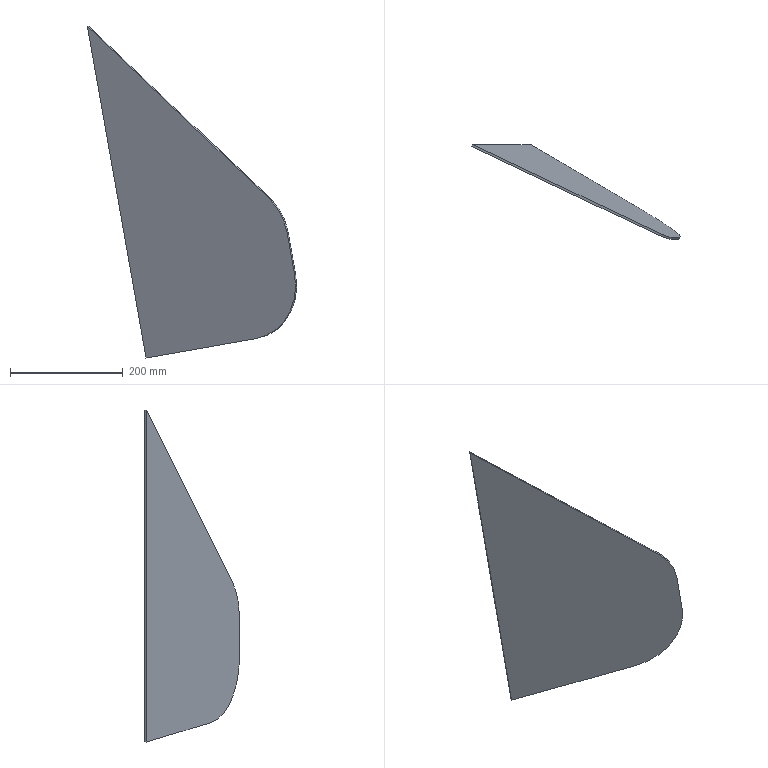Part | STEP file | floating channel left front section | 1 solid | 8 faces | box 372.026 x 168.494 x 590.246 mm | volume 526748 mm3 | plane 6 | cylinder 2 | commonest cylinder face diameters 200 x2
STEP:
#1=CARTESIAN_POINT('',(0.,0.,0.));
#2=DIRECTION('',(0.,0.,1.));
#3=DIRECTION('',(1.,0.,0.));
#4=AXIS2_PLACEMENT_3D('',#1,#2,#3);
#5=CARTESIAN_POINT('',(2326.268,155.426,-236.438));
#6=VERTEX_POINT('',#5);
#7=CARTESIAN_POINT('',(2358.025,143.435,-296.806));
#8=VERTEX_POINT('',#7);
#9=CARTESIAN_POINT('',(2272.743,193.435,-311.873));
#10=DIRECTION('',(0.4924,0.866,0.08699));
#11=DIRECTION('',(0.8693,-0.4942,0.));
#12=AXIS2_PLACEMENT_3D('',#9,#10,#11);
#13=CIRCLE('',#12,100.);
#14=CARTESIAN_POINT('',(2272.743,193.435,-311.873));
#15=DIRECTION('',(-0.4924,-0.866,-0.08699));
#16=DIRECTION('',(-0.8693,0.4942,0.));
#17=AXIS2_PLACEMENT_3D('',#14,#15,#16);
#18=CYLINDRICAL_SURFACE('',#17,100.);
#19=CARTESIAN_POINT('',(9.425,0.));
#20=DIRECTION('',(-1.,0.));
#21=VECTOR('',#20,1.);
#22=LINE('',#19,#21);
#23=(GEOMETRIC_REPRESENTATION_CONTEXT(2)PARAMETRIC_REPRESENTATION_CONTEXT()REPRESENTATION_CONTEXT('',''));
#24=DEFINITIONAL_REPRESENTATION('',(#22),#23);
#25=PCURVE('',#18,#24);
#26=CARTESIAN_POINT('',(620.113,1090.7,109.555));
#27=DIRECTION('',(-0.4924,-0.866,-0.08699));
#28=DIRECTION('',(-0.8693,0.4942,0.));
#29=AXIS2_PLACEMENT_3D('',#26,#27,#28);
#30=PLANE('',#29);
#31=CARTESIAN_POINT('',(-1980.138,423.031));
#32=CARTESIAN_POINT('',(-1980.138,596.236));
#33=CARTESIAN_POINT('',(-1830.138,509.633));
#34=CARTESIAN_POINT('',(-1680.138,423.031));
#35=CARTESIAN_POINT('',(-1830.138,336.428));
#36=CARTESIAN_POINT('',(-1980.138,249.826));
#37=CARTESIAN_POINT('',(-1980.138,423.031));
#38=(BOUNDED_CURVE()B_SPLINE_CURVE(2,(#31,#32,#33,#34,#35,#36,#37),.UNSPECIFIED.,.T.,.F.)B_SPLINE_CURVE_WITH_KNOTS((1,2,2,2,2,1),(-2.094,0.,2.094,4.189,6.283,8.378),.UNSPECIFIED.)CURVE()GEOMETRIC_REPRESENTATION_ITEM()RATIONAL_B_SPLINE_CURVE((1.,0.5,1.,0.5,1.,0.5,1.))REPRESENTATION_ITEM(''));
#39=(GEOMETRIC_REPRESENTATION_CONTEXT(2)PARAMETRIC_REPRESENTATION_CONTEXT()REPRESENTATION_CONTEXT('',''));
#40=DEFINITIONAL_REPRESENTATION('',(#38),#39);
#41=PCURVE('',#30,#40);
#42=SURFACE_CURVE('',#13,(#25,#41),.PCURVE_S1.);
#43=EDGE_CURVE('',#6,#8,#42,.T.);
#44=ORIENTED_EDGE('',*,*,#43,.F.);
#45=CARTESIAN_POINT('',(2324.298,151.962,-236.786));
#46=VERTEX_POINT('',#45);
#47=CARTESIAN_POINT('',(2326.268,155.426,-236.438));
#48=DIRECTION('',(0.4924,0.866,0.08699));
#49=VECTOR('',#48,1.);
#50=LINE('',#47,#49);
#51=CARTESIAN_POINT('',(4.001,0.));
#52=DIRECTION('',(0.,-1.));
#53=VECTOR('',#52,1.);
#54=LINE('',#51,#53);
#55=(GEOMETRIC_REPRESENTATION_CONTEXT(2)PARAMETRIC_REPRESENTATION_CONTEXT()REPRESENTATION_CONTEXT('',''));
#56=DEFINITIONAL_REPRESENTATION('',(#54),#55);
#57=PCURVE('',#18,#56);
#58=CARTESIAN_POINT('',(2002.94,308.464,70.087));
#59=DIRECTION('',(-0.5352,0.3801,-0.7544));
#60=DIRECTION('',(0.8156,0.,-0.5787));
#61=AXIS2_PLACEMENT_3D('',#58,#59,#60);
#62=PLANE('',#61);
#63=CARTESIAN_POINT('',(441.071,165.455));
#64=DIRECTION('',(0.3512,-0.9363));
#65=VECTOR('',#64,1.);
#66=LINE('',#63,#65);
#67=(GEOMETRIC_REPRESENTATION_CONTEXT(2)PARAMETRIC_REPRESENTATION_CONTEXT()REPRESENTATION_CONTEXT('',''));
#68=DEFINITIONAL_REPRESENTATION('',(#66),#67);
#69=PCURVE('',#62,#68);
#70=SURFACE_CURVE('',#50,(#57,#69),.PCURVE_S1.);
#71=EDGE_CURVE('',#46,#6,#70,.T.);
#72=ORIENTED_EDGE('',*,*,#71,.F.);
#73=CARTESIAN_POINT('',(2356.056,139.97,-297.154));
#74=VERTEX_POINT('',#73);
#75=CARTESIAN_POINT('',(2270.774,189.97,-312.221));
#76=DIRECTION('',(-0.4924,-0.866,-0.08699));
#77=DIRECTION('',(0.8693,-0.4942,0.));
#78=AXIS2_PLACEMENT_3D('',#75,#76,#77);
#79=CIRCLE('',#78,100.);
#80=CARTESIAN_POINT('',(3.142,4.));
#81=DIRECTION('',(1.,0.));
#82=VECTOR('',#81,1.);
#83=LINE('',#80,#82);
#84=(GEOMETRIC_REPRESENTATION_CONTEXT(2)PARAMETRIC_REPRESENTATION_CONTEXT()REPRESENTATION_CONTEXT('',''));
#85=DEFINITIONAL_REPRESENTATION('',(#83),#84);
#86=PCURVE('',#18,#85);
#87=CARTESIAN_POINT('',(618.144,1087.236,109.207));
#88=DIRECTION('',(-0.4924,-0.866,-0.08699));
#89=DIRECTION('',(-0.8693,0.4942,0.));
#90=AXIS2_PLACEMENT_3D('',#87,#88,#89);
#91=PLANE('',#90);
#92=CARTESIAN_POINT('',(-1880.138,423.031));
#93=DIRECTION('',(-1.,0.));
#94=AXIS2_PLACEMENT_2D('',#92,#93);
#95=CIRCLE('',#94,100.);
#96=(GEOMETRIC_REPRESENTATION_CONTEXT(2)PARAMETRIC_REPRESENTATION_CONTEXT()REPRESENTATION_CONTEXT('',''));
#97=DEFINITIONAL_REPRESENTATION('',(#95),#96);
#98=PCURVE('',#91,#97);
#99=SURFACE_CURVE('',#79,(#86,#98),.PCURVE_S1.);
#100=EDGE_CURVE('',#74,#46,#99,.T.);
#101=ORIENTED_EDGE('',*,*,#100,.F.);
#102=CARTESIAN_POINT('',(2358.025,143.435,-296.806));
#103=DIRECTION('',(-0.4924,-0.866,-0.08699));
#104=VECTOR('',#103,1.);
#105=LINE('',#102,#104);
#106=CARTESIAN_POINT('',(3.293,0.));
#107=DIRECTION('',(0.,1.));
#108=VECTOR('',#107,1.);
#109=LINE('',#106,#108);
#110=(GEOMETRIC_REPRESENTATION_CONTEXT(2)PARAMETRIC_REPRESENTATION_CONTEXT()REPRESENTATION_CONTEXT('',''));
#111=DEFINITIONAL_REPRESENTATION('',(#109),#110);
#112=PCURVE('',#18,#111);
#113=CARTESIAN_POINT('',(2351.603,143.435,-260.456));
#114=DIRECTION('',(-0.8528,0.5,-0.1507));
#115=DIRECTION('',(0.5058,0.8627,0.));
#116=AXIS2_PLACEMENT_3D('',#113,#114,#115);
#117=PLANE('',#116);
#118=CARTESIAN_POINT('',(3.248,36.77));
#119=DIRECTION('',(-0.9961,0.08799));
#120=VECTOR('',#119,1.);
#121=LINE('',#118,#120);
#122=(GEOMETRIC_REPRESENTATION_CONTEXT(2)PARAMETRIC_REPRESENTATION_CONTEXT()REPRESENTATION_CONTEXT('',''));
#123=DEFINITIONAL_REPRESENTATION('',(#121),#122);
#124=PCURVE('',#117,#123);
#125=SURFACE_CURVE('',#105,(#112,#124),.PCURVE_S1.);
#126=EDGE_CURVE('',#8,#74,#125,.T.);
#127=ORIENTED_EDGE('',*,*,#126,.F.);
#128=EDGE_LOOP('',(#44,#72,#101,#127));
#129=FACE_BOUND('',#128,.T.);
#130=ADVANCED_FACE('',(#129),#18,.T.);
#131=CARTESIAN_POINT('',(2371.24,143.435,-371.607));
#132=VERTEX_POINT('',#131);
#133=CARTESIAN_POINT('',(2303.356,193.435,-485.148));
#134=VERTEX_POINT('',#133);
#135=CARTESIAN_POINT('',(2285.958,193.435,-386.673));
#136=DIRECTION('',(0.4924,0.866,0.08699));
#137=DIRECTION('',(0.8693,-0.4942,0.));
#138=AXIS2_PLACEMENT_3D('',#135,#136,#137);
#139=CIRCLE('',#138,100.);
#140=CARTESIAN_POINT('',(2285.958,193.435,-386.673));
#141=DIRECTION('',(-0.4924,-0.866,-0.08699));
#142=DIRECTION('',(-0.8693,0.4942,0.));
#143=AXIS2_PLACEMENT_3D('',#140,#141,#142);
#144=CYLINDRICAL_SURFACE('',#143,100.);
#145=CARTESIAN_POINT('',(9.425,0.));
#146=DIRECTION('',(-1.,0.));
#147=VECTOR('',#146,1.);
#148=LINE('',#145,#147);
#149=(GEOMETRIC_REPRESENTATION_CONTEXT(2)PARAMETRIC_REPRESENTATION_CONTEXT()REPRESENTATION_CONTEXT('',''));
#150=DEFINITIONAL_REPRESENTATION('',(#148),#149);
#151=PCURVE('',#144,#150);
#152=CARTESIAN_POINT('',(-1991.626,498.116));
#153=CARTESIAN_POINT('',(-1991.626,671.321));
#154=CARTESIAN_POINT('',(-1841.626,584.719));
#155=CARTESIAN_POINT('',(-1691.626,498.116));
#156=CARTESIAN_POINT('',(-1841.626,411.514));
#157=CARTESIAN_POINT('',(-1991.626,324.911));
#158=CARTESIAN_POINT('',(-1991.626,498.116));
#159=(BOUNDED_CURVE()B_SPLINE_CURVE(2,(#152,#153,#154,#155,#156,#157,#158),.UNSPECIFIED.,.T.,.F.)B_SPLINE_CURVE_WITH_KNOTS((1,2,2,2,2,1),(-2.094,0.,2.094,4.189,6.283,8.378),.UNSPECIFIED.)CURVE()GEOMETRIC_REPRESENTATION_ITEM()RATIONAL_B_SPLINE_CURVE((1.,0.5,1.,0.5,1.,0.5,1.))REPRESENTATION_ITEM(''));
#160=(GEOMETRIC_REPRESENTATION_CONTEXT(2)PARAMETRIC_REPRESENTATION_CONTEXT()REPRESENTATION_CONTEXT('',''));
#161=DEFINITIONAL_REPRESENTATION('',(#159),#160);
#162=PCURVE('',#30,#161);
#163=SURFACE_CURVE('',#139,(#151,#162),.PCURVE_S1.);
#164=EDGE_CURVE('',#132,#134,#163,.T.);
#165=ORIENTED_EDGE('',*,*,#164,.F.);
#166=CARTESIAN_POINT('',(2369.271,139.97,-371.955));
#167=VERTEX_POINT('',#166);
#168=CARTESIAN_POINT('',(2371.24,143.435,-371.607));
#169=DIRECTION('',(0.4924,0.866,0.08699));
#170=VECTOR('',#169,1.);
#171=LINE('',#168,#170);
#172=CARTESIAN_POINT('',(3.293,0.));
#173=DIRECTION('',(0.,-1.));
#174=VECTOR('',#173,1.);
#175=LINE('',#172,#174);
#176=(GEOMETRIC_REPRESENTATION_CONTEXT(2)PARAMETRIC_REPRESENTATION_CONTEXT()REPRESENTATION_CONTEXT('',''));
#177=DEFINITIONAL_REPRESENTATION('',(#175),#176);
#178=PCURVE('',#144,#177);
#179=CARTESIAN_POINT('',(9.932,112.434));
#180=DIRECTION('',(0.9961,-0.08799));
#181=VECTOR('',#180,1.);
#182=LINE('',#179,#181);
#183=(GEOMETRIC_REPRESENTATION_CONTEXT(2)PARAMETRIC_REPRESENTATION_CONTEXT()REPRESENTATION_CONTEXT('',''));
#184=DEFINITIONAL_REPRESENTATION('',(#182),#183);
#185=PCURVE('',#117,#184);
#186=SURFACE_CURVE('',#171,(#178,#185),.PCURVE_S1.);
#187=EDGE_CURVE('',#167,#132,#186,.T.);
#188=ORIENTED_EDGE('',*,*,#187,.F.);
#189=CARTESIAN_POINT('',(2301.386,189.97,-485.496));
#190=VERTEX_POINT('',#189);
#191=CARTESIAN_POINT('',(2283.989,189.97,-387.021));
#192=DIRECTION('',(-0.4924,-0.866,-0.08699));
#193=DIRECTION('',(0.8693,-0.4942,0.));
#194=AXIS2_PLACEMENT_3D('',#191,#192,#193);
#195=CIRCLE('',#194,100.);
#196=CARTESIAN_POINT('',(-3.142,4.));
#197=DIRECTION('',(1.,0.));
#198=VECTOR('',#197,1.);
#199=LINE('',#196,#198);
#200=(GEOMETRIC_REPRESENTATION_CONTEXT(2)PARAMETRIC_REPRESENTATION_CONTEXT()REPRESENTATION_CONTEXT('',''));
#201=DEFINITIONAL_REPRESENTATION('',(#199),#200);
#202=PCURVE('',#144,#201);
#203=CARTESIAN_POINT('',(-1891.626,498.116));
#204=DIRECTION('',(-1.,0.));
#205=AXIS2_PLACEMENT_2D('',#203,#204);
#206=CIRCLE('',#205,100.);
#207=(GEOMETRIC_REPRESENTATION_CONTEXT(2)PARAMETRIC_REPRESENTATION_CONTEXT()REPRESENTATION_CONTEXT('',''));
#208=DEFINITIONAL_REPRESENTATION('',(#206),#207);
#209=PCURVE('',#91,#208);
#210=SURFACE_CURVE('',#195,(#202,#209),.PCURVE_S1.);
#211=EDGE_CURVE('',#190,#167,#210,.T.);
#212=ORIENTED_EDGE('',*,*,#211,.F.);
#213=CARTESIAN_POINT('',(2303.356,193.435,-485.148));
#214=DIRECTION('',(-0.4924,-0.866,-0.08699));
#215=VECTOR('',#214,1.);
#216=LINE('',#213,#215);
#217=CARTESIAN_POINT('',(1.723,0.));
#218=DIRECTION('',(0.,1.));
#219=VECTOR('',#218,1.);
#220=LINE('',#217,#219);
#221=(GEOMETRIC_REPRESENTATION_CONTEXT(2)PARAMETRIC_REPRESENTATION_CONTEXT()REPRESENTATION_CONTEXT('',''));
#222=DEFINITIONAL_REPRESENTATION('',(#220),#221);
#223=PCURVE('',#144,#222);
#224=CARTESIAN_POINT('',(2388.637,143.435,-470.082));
#225=DIRECTION('',(-0.174,0.,0.9848));
#226=DIRECTION('',(-0.9848,0.,-0.174));
#227=AXIS2_PLACEMENT_3D('',#224,#225,#226);
#228=PLANE('',#227);
#229=CARTESIAN_POINT('',(86.603,-50.));
#230=DIRECTION('',(0.5,0.866));
#231=VECTOR('',#230,1.);
#232=LINE('',#229,#231);
#233=(GEOMETRIC_REPRESENTATION_CONTEXT(2)PARAMETRIC_REPRESENTATION_CONTEXT()REPRESENTATION_CONTEXT('',''));
#234=DEFINITIONAL_REPRESENTATION('',(#232),#233);
#235=PCURVE('',#228,#234);
#236=SURFACE_CURVE('',#216,(#223,#235),.PCURVE_S1.);
#237=EDGE_CURVE('',#134,#190,#236,.T.);
#238=ORIENTED_EDGE('',*,*,#237,.F.);
#239=EDGE_LOOP('',(#165,#188,#212,#238));
#240=FACE_BOUND('',#239,.T.);
#241=ADVANCED_FACE('',(#240),#144,.T.);
#242=CARTESIAN_POINT('',(2349.634,139.97,-260.804));
#243=DIRECTION('',(0.174,0.,-0.9848));
#244=VECTOR('',#243,1.);
#245=LINE('',#242,#244);
#246=CARTESIAN_POINT('',(-1973.405,371.419));
#247=DIRECTION('',(-0.1512,0.9885));
#248=VECTOR('',#247,1.);
#249=LINE('',#246,#248);
#250=(GEOMETRIC_REPRESENTATION_CONTEXT(2)PARAMETRIC_REPRESENTATION_CONTEXT()REPRESENTATION_CONTEXT('',''));
#251=DEFINITIONAL_REPRESENTATION('',(#249),#250);
#252=PCURVE('',#91,#251);
#253=CARTESIAN_POINT('',(-3.984,0.352));
#254=DIRECTION('',(0.08799,0.9961));
#255=VECTOR('',#254,1.);
#256=LINE('',#253,#255);
#257=(GEOMETRIC_REPRESENTATION_CONTEXT(2)PARAMETRIC_REPRESENTATION_CONTEXT()REPRESENTATION_CONTEXT('',''));
#258=DEFINITIONAL_REPRESENTATION('',(#256),#257);
#259=PCURVE('',#117,#258);
#260=SURFACE_CURVE('',#245,(#252,#259),.PCURVE_S1.);
#261=EDGE_CURVE('',#74,#167,#260,.T.);
#262=ORIENTED_EDGE('',*,*,#261,.F.);
#263=ORIENTED_EDGE('',*,*,#100,.T.);
#264=CARTESIAN_POINT('',(2000.971,305.,69.739));
#265=VERTEX_POINT('',#264);
#266=CARTESIAN_POINT('',(2000.971,305.,69.739));
#267=DIRECTION('',(0.6864,-0.3249,-0.6507));
#268=VECTOR('',#267,1.);
#269=LINE('',#266,#268);
#270=CARTESIAN_POINT('',(-1588.739,39.618));
#271=DIRECTION('',(-0.7572,0.6532));
#272=VECTOR('',#271,1.);
#273=LINE('',#270,#272);
#274=(GEOMETRIC_REPRESENTATION_CONTEXT(2)PARAMETRIC_REPRESENTATION_CONTEXT()REPRESENTATION_CONTEXT('',''));
#275=DEFINITIONAL_REPRESENTATION('',(#273),#274);
#276=PCURVE('',#91,#275);
#277=CARTESIAN_POINT('',(-1.405,3.745));
#278=DIRECTION('',(0.9363,0.3512));
#279=VECTOR('',#278,1.);
#280=LINE('',#277,#279);
#281=(GEOMETRIC_REPRESENTATION_CONTEXT(2)PARAMETRIC_REPRESENTATION_CONTEXT()REPRESENTATION_CONTEXT('',''));
#282=DEFINITIONAL_REPRESENTATION('',(#280),#281);
#283=PCURVE('',#62,#282);
#284=SURFACE_CURVE('',#269,(#276,#283),.PCURVE_S1.);
#285=EDGE_CURVE('',#265,#46,#284,.T.);
#286=ORIENTED_EDGE('',*,*,#285,.F.);
#287=CARTESIAN_POINT('',(2105.187,305.,-520.159));
#288=VERTEX_POINT('',#287);
#289=CARTESIAN_POINT('',(2105.187,305.,-520.159));
#290=DIRECTION('',(-0.174,0.,0.9848));
#291=VECTOR('',#290,1.);
#292=LINE('',#289,#291);
#293=CARTESIAN_POINT('',(-1679.337,631.76));
#294=DIRECTION('',(0.1512,-0.9885));
#295=VECTOR('',#294,1.);
#296=LINE('',#293,#295);
#297=(GEOMETRIC_REPRESENTATION_CONTEXT(2)PARAMETRIC_REPRESENTATION_CONTEXT()REPRESENTATION_CONTEXT('',''));
#298=DEFINITIONAL_REPRESENTATION('',(#296),#297);
#299=PCURVE('',#91,#298);
#300=CARTESIAN_POINT('',(2107.157,308.464,-519.811));
#301=DIRECTION('',(0.8528,-0.5,0.1507));
#302=DIRECTION('',(-0.5058,-0.8627,0.));
#303=AXIS2_PLACEMENT_3D('',#300,#301,#302);
#304=PLANE('',#303);
#305=CARTESIAN_POINT('',(3.984,0.352));
#306=DIRECTION('',(0.08799,-0.9961));
#307=VECTOR('',#306,1.);
#308=LINE('',#305,#307);
#309=(GEOMETRIC_REPRESENTATION_CONTEXT(2)PARAMETRIC_REPRESENTATION_CONTEXT()REPRESENTATION_CONTEXT('',''));
#310=DEFINITIONAL_REPRESENTATION('',(#308),#309);
#311=PCURVE('',#304,#310);
#312=SURFACE_CURVE('',#292,(#299,#311),.PCURVE_S1.);
#313=EDGE_CURVE('',#288,#265,#312,.T.);
#314=ORIENTED_EDGE('',*,*,#313,.F.);
#315=CARTESIAN_POINT('',(2386.668,139.97,-470.43));
#316=DIRECTION('',(-0.8528,0.5,-0.1507));
#317=VECTOR('',#316,1.);
#318=LINE('',#315,#317);
#319=CARTESIAN_POINT('',(-2005.6,581.842));
#320=DIRECTION('',(0.9885,0.1512));
#321=VECTOR('',#320,1.);
#322=LINE('',#319,#321);
#323=(GEOMETRIC_REPRESENTATION_CONTEXT(2)PARAMETRIC_REPRESENTATION_CONTEXT()REPRESENTATION_CONTEXT('',''));
#324=DEFINITIONAL_REPRESENTATION('',(#322),#323);
#325=PCURVE('',#91,#324);
#326=CARTESIAN_POINT('',(2.,3.464));
#327=DIRECTION('',(0.866,-0.5));
#328=VECTOR('',#327,1.);
#329=LINE('',#326,#328);
#330=(GEOMETRIC_REPRESENTATION_CONTEXT(2)PARAMETRIC_REPRESENTATION_CONTEXT()REPRESENTATION_CONTEXT('',''));
#331=DEFINITIONAL_REPRESENTATION('',(#329),#330);
#332=PCURVE('',#228,#331);
#333=SURFACE_CURVE('',#318,(#325,#332),.PCURVE_S1.);
#334=EDGE_CURVE('',#190,#288,#333,.T.);
#335=ORIENTED_EDGE('',*,*,#334,.F.);
#336=ORIENTED_EDGE('',*,*,#211,.T.);
#337=EDGE_LOOP('',(#262,#263,#286,#314,#335,#336));
#338=FACE_BOUND('',#337,.T.);
#339=ADVANCED_FACE('',(#338),#91,.T.);
#340=CARTESIAN_POINT('',(2002.94,308.464,70.087));
#341=VERTEX_POINT('',#340);
#342=CARTESIAN_POINT('',(2002.94,308.464,70.087));
#343=DIRECTION('',(0.6864,-0.3249,-0.6507));
#344=VECTOR('',#343,1.);
#345=LINE('',#342,#344);
#346=CARTESIAN_POINT('',(-1588.739,39.618));
#347=DIRECTION('',(-0.7572,0.6532));
#348=VECTOR('',#347,1.);
#349=LINE('',#346,#348);
#350=(GEOMETRIC_REPRESENTATION_CONTEXT(2)PARAMETRIC_REPRESENTATION_CONTEXT()REPRESENTATION_CONTEXT('',''));
#351=DEFINITIONAL_REPRESENTATION('',(#349),#350);
#352=PCURVE('',#30,#351);
#353=CARTESIAN_POINT('',(0.,0.));
#354=DIRECTION('',(0.9363,0.3512));
#355=VECTOR('',#354,1.);
#356=LINE('',#353,#355);
#357=(GEOMETRIC_REPRESENTATION_CONTEXT(2)PARAMETRIC_REPRESENTATION_CONTEXT()REPRESENTATION_CONTEXT('',''));
#358=DEFINITIONAL_REPRESENTATION('',(#356),#357);
#359=PCURVE('',#62,#358);
#360=SURFACE_CURVE('',#345,(#352,#359),.PCURVE_S1.);
#361=EDGE_CURVE('',#341,#6,#360,.T.);
#362=ORIENTED_EDGE('',*,*,#361,.T.);
#363=ORIENTED_EDGE('',*,*,#43,.T.);
#364=CARTESIAN_POINT('',(2351.603,143.435,-260.456));
#365=DIRECTION('',(0.174,0.,-0.9848));
#366=VECTOR('',#365,1.);
#367=LINE('',#364,#366);
#368=CARTESIAN_POINT('',(-1973.405,371.419));
#369=DIRECTION('',(-0.1512,0.9885));
#370=VECTOR('',#369,1.);
#371=LINE('',#368,#370);
#372=(GEOMETRIC_REPRESENTATION_CONTEXT(2)PARAMETRIC_REPRESENTATION_CONTEXT()REPRESENTATION_CONTEXT('',''));
#373=DEFINITIONAL_REPRESENTATION('',(#371),#372);
#374=PCURVE('',#30,#373);
#375=CARTESIAN_POINT('',(0.,0.));
#376=DIRECTION('',(0.08799,0.9961));
#377=VECTOR('',#376,1.);
#378=LINE('',#375,#377);
#379=(GEOMETRIC_REPRESENTATION_CONTEXT(2)PARAMETRIC_REPRESENTATION_CONTEXT()REPRESENTATION_CONTEXT('',''));
#380=DEFINITIONAL_REPRESENTATION('',(#378),#379);
#381=PCURVE('',#117,#380);
#382=SURFACE_CURVE('',#367,(#374,#381),.PCURVE_S1.);
#383=EDGE_CURVE('',#8,#132,#382,.T.);
#384=ORIENTED_EDGE('',*,*,#383,.T.);
#385=ORIENTED_EDGE('',*,*,#164,.T.);
#386=CARTESIAN_POINT('',(2107.157,308.464,-519.811));
#387=VERTEX_POINT('',#386);
#388=CARTESIAN_POINT('',(2388.637,143.435,-470.082));
#389=DIRECTION('',(-0.8528,0.5,-0.1507));
#390=VECTOR('',#389,1.);
#391=LINE('',#388,#390);
#392=CARTESIAN_POINT('',(-2005.6,581.842));
#393=DIRECTION('',(0.9885,0.1512));
#394=VECTOR('',#393,1.);
#395=LINE('',#392,#394);
#396=(GEOMETRIC_REPRESENTATION_CONTEXT(2)PARAMETRIC_REPRESENTATION_CONTEXT()REPRESENTATION_CONTEXT('',''));
#397=DEFINITIONAL_REPRESENTATION('',(#395),#396);
#398=PCURVE('',#30,#397);
#399=CARTESIAN_POINT('',(0.,0.));
#400=DIRECTION('',(0.866,-0.5));
#401=VECTOR('',#400,1.);
#402=LINE('',#399,#401);
#403=(GEOMETRIC_REPRESENTATION_CONTEXT(2)PARAMETRIC_REPRESENTATION_CONTEXT()REPRESENTATION_CONTEXT('',''));
#404=DEFINITIONAL_REPRESENTATION('',(#402),#403);
#405=PCURVE('',#228,#404);
#406=SURFACE_CURVE('',#391,(#398,#405),.PCURVE_S1.);
#407=EDGE_CURVE('',#134,#387,#406,.T.);
#408=ORIENTED_EDGE('',*,*,#407,.T.);
#409=CARTESIAN_POINT('',(2072.53,308.464,-323.813));
#410=DIRECTION('',(-0.174,0.,0.9848));
#411=VECTOR('',#410,1.);
#412=LINE('',#409,#411);
#413=CARTESIAN_POINT('',(-1649.235,435.017));
#414=DIRECTION('',(0.1512,-0.9885));
#415=VECTOR('',#414,1.);
#416=LINE('',#413,#415);
#417=(GEOMETRIC_REPRESENTATION_CONTEXT(2)PARAMETRIC_REPRESENTATION_CONTEXT()REPRESENTATION_CONTEXT('',''));
#418=DEFINITIONAL_REPRESENTATION('',(#416),#417);
#419=PCURVE('',#30,#418);
#420=CARTESIAN_POINT('',(17.513,-198.261));
#421=DIRECTION('',(0.08799,-0.9961));
#422=VECTOR('',#421,1.);
#423=LINE('',#420,#422);
#424=(GEOMETRIC_REPRESENTATION_CONTEXT(2)PARAMETRIC_REPRESENTATION_CONTEXT()REPRESENTATION_CONTEXT('',''));
#425=DEFINITIONAL_REPRESENTATION('',(#423),#424);
#426=PCURVE('',#304,#425);
#427=SURFACE_CURVE('',#412,(#419,#426),.PCURVE_S1.);
#428=EDGE_CURVE('',#387,#341,#427,.T.);
#429=ORIENTED_EDGE('',*,*,#428,.T.);
#430=EDGE_LOOP('',(#362,#363,#384,#385,#408,#429));
#431=FACE_BOUND('',#430,.T.);
#432=ADVANCED_FACE('',(#431),#30,.F.);
#433=ORIENTED_EDGE('',*,*,#313,.T.);
#434=CARTESIAN_POINT('',(2002.94,308.464,70.087));
#435=DIRECTION('',(-0.4924,-0.866,-0.08699));
#436=VECTOR('',#435,1.);
#437=LINE('',#434,#436);
#438=CARTESIAN_POINT('',(52.71,-596.709));
#439=DIRECTION('',(0.9961,0.08799));
#440=VECTOR('',#439,1.);
#441=LINE('',#438,#440);
#442=(GEOMETRIC_REPRESENTATION_CONTEXT(2)PARAMETRIC_REPRESENTATION_CONTEXT()REPRESENTATION_CONTEXT('',''));
#443=DEFINITIONAL_REPRESENTATION('',(#441),#442);
#444=PCURVE('',#304,#443);
#445=CARTESIAN_POINT('',(0.,0.));
#446=DIRECTION('',(-0.3512,0.9363));
#447=VECTOR('',#446,1.);
#448=LINE('',#445,#447);
#449=(GEOMETRIC_REPRESENTATION_CONTEXT(2)PARAMETRIC_REPRESENTATION_CONTEXT()REPRESENTATION_CONTEXT('',''));
#450=DEFINITIONAL_REPRESENTATION('',(#448),#449);
#451=PCURVE('',#62,#450);
#452=SURFACE_CURVE('',#437,(#444,#451),.PCURVE_S1.);
#453=EDGE_CURVE('',#341,#265,#452,.T.);
#454=ORIENTED_EDGE('',*,*,#453,.F.);
#455=ORIENTED_EDGE('',*,*,#428,.F.);
#456=CARTESIAN_POINT('',(2107.157,308.464,-519.811));
#457=DIRECTION('',(-0.4924,-0.866,-0.08699));
#458=VECTOR('',#457,1.);
#459=LINE('',#456,#458);
#460=CARTESIAN_POINT('',(0.,0.));
#461=DIRECTION('',(0.9961,0.08799));
#462=VECTOR('',#461,1.);
#463=LINE('',#460,#462);
#464=(GEOMETRIC_REPRESENTATION_CONTEXT(2)PARAMETRIC_REPRESENTATION_CONTEXT()REPRESENTATION_CONTEXT('',''));
#465=DEFINITIONAL_REPRESENTATION('',(#463),#464);
#466=PCURVE('',#304,#465);
#467=CARTESIAN_POINT('',(285.84,-165.03));
#468=DIRECTION('',(0.5,0.866));
#469=VECTOR('',#468,1.);
#470=LINE('',#467,#469);
#471=(GEOMETRIC_REPRESENTATION_CONTEXT(2)PARAMETRIC_REPRESENTATION_CONTEXT()REPRESENTATION_CONTEXT('',''));
#472=DEFINITIONAL_REPRESENTATION('',(#470),#471);
#473=PCURVE('',#228,#472);
#474=SURFACE_CURVE('',#459,(#466,#473),.PCURVE_S1.);
#475=EDGE_CURVE('',#387,#288,#474,.T.);
#476=ORIENTED_EDGE('',*,*,#475,.T.);
#477=EDGE_LOOP('',(#433,#454,#455,#476));
#478=FACE_BOUND('',#477,.T.);
#479=ADVANCED_FACE('',(#478),#304,.F.);
#480=ORIENTED_EDGE('',*,*,#407,.F.);
#481=ORIENTED_EDGE('',*,*,#237,.T.);
#482=ORIENTED_EDGE('',*,*,#334,.T.);
#483=ORIENTED_EDGE('',*,*,#475,.F.);
#484=EDGE_LOOP('',(#480,#481,#482,#483));
#485=FACE_BOUND('',#484,.T.);
#486=ADVANCED_FACE('',(#485),#228,.F.);
#487=ORIENTED_EDGE('',*,*,#383,.F.);
#488=ORIENTED_EDGE('',*,*,#126,.T.);
#489=ORIENTED_EDGE('',*,*,#261,.T.);
#490=ORIENTED_EDGE('',*,*,#187,.T.);
#491=EDGE_LOOP('',(#487,#488,#489,#490));
#492=FACE_BOUND('',#491,.T.);
#493=ADVANCED_FACE('',(#492),#117,.F.);
#494=ORIENTED_EDGE('',*,*,#285,.T.);
#495=ORIENTED_EDGE('',*,*,#71,.T.);
#496=ORIENTED_EDGE('',*,*,#361,.F.);
#497=ORIENTED_EDGE('',*,*,#453,.T.);
#498=EDGE_LOOP('',(#494,#495,#496,#497));
#499=FACE_BOUND('',#498,.T.);
#500=ADVANCED_FACE('',(#499),#62,.F.);
#501=CLOSED_SHELL('',(#130,#241,#339,#432,#479,#486,#493,#500));
#502=MANIFOLD_SOLID_BREP('',#501);
#503=(LENGTH_UNIT()NAMED_UNIT(*)SI_UNIT(.MILLI.,.METRE.));
#504=UNCERTAINTY_MEASURE_WITH_UNIT(LENGTH_MEASURE(0.0000001),#503,'','');
#505=(NAMED_UNIT(*)PLANE_ANGLE_UNIT()SI_UNIT($,.RADIAN.));
#506=(NAMED_UNIT(*)SI_UNIT($,.STERADIAN.)SOLID_ANGLE_UNIT());
#507=(GEOMETRIC_REPRESENTATION_CONTEXT(3)GLOBAL_UNCERTAINTY_ASSIGNED_CONTEXT((#504))GLOBAL_UNIT_ASSIGNED_CONTEXT((#503,#505,#506))REPRESENTATION_CONTEXT('',''));
#508=ADVANCED_BREP_SHAPE_REPRESENTATION('',(#4,#502),#507);